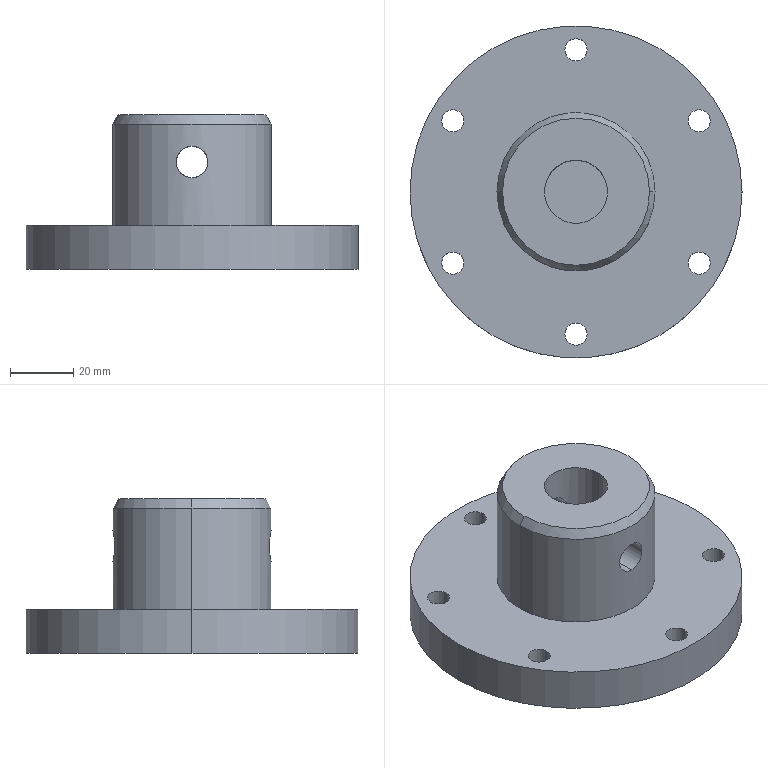Part | SolidWorks | features ICE 2, Chamfer 1, Extrusion 1 | 1 solid | 28 faces | box 105 x 105 x 49 mm | volume 172934 mm3 | cylinder 22 | plane 4 | cone 2 | commonest cylinder face diameters 7 x12 10 x4 20 x2 50 x2 105 x2
STEP:
#1=CARTESIAN_POINT('',(23.268,0.,49.));
#2=VERTEX_POINT('',#1);
#3=CARTESIAN_POINT('',(-23.268,0.,49.));
#4=VERTEX_POINT('',#3);
#5=CARTESIAN_POINT('',(0.,0.,49.));
#6=DIRECTION('',(0.,0.,1.));
#7=DIRECTION('',(1.,0.,0.));
#8=AXIS2_PLACEMENT_3D('',#5,#6,#7);
#9=CIRCLE('',#8,23.268);
#10=EDGE_CURVE('',#2,#4,#9,.T.);
#11=ORIENTED_EDGE('',*,*,#10,.F.);
#12=CARTESIAN_POINT('',(25.,0.,46.));
#13=VERTEX_POINT('',#12);
#14=CARTESIAN_POINT('',(23.268,0.,49.));
#15=DIRECTION('',(0.5,0.,-0.866));
#16=VECTOR('',#15,1000.);
#17=LINE('',#14,#16);
#18=EDGE_CURVE('',#2,#13,#17,.T.);
#19=ORIENTED_EDGE('',*,*,#18,.T.);
#20=CARTESIAN_POINT('',(-25.,0.,46.));
#21=VERTEX_POINT('',#20);
#22=CARTESIAN_POINT('',(0.,0.,46.));
#23=DIRECTION('',(0.,0.,-1.));
#24=DIRECTION('',(1.,0.,0.));
#25=AXIS2_PLACEMENT_3D('',#22,#23,#24);
#26=CIRCLE('',#25,25.);
#27=EDGE_CURVE('',#21,#13,#26,.T.);
#28=ORIENTED_EDGE('',*,*,#27,.F.);
#29=CARTESIAN_POINT('',(-23.268,0.,49.));
#30=DIRECTION('',(-0.5,0.,-0.866));
#31=VECTOR('',#30,1000.);
#32=LINE('',#29,#31);
#33=EDGE_CURVE('',#4,#21,#32,.T.);
#34=ORIENTED_EDGE('',*,*,#33,.F.);
#35=EDGE_LOOP('',(#11,#19,#28,#34));
#36=FACE_OUTER_BOUND('',#35,.T.);
#37=CARTESIAN_POINT('',(0.,0.,49.));
#38=DIRECTION('',(0.,0.,-1.));
#39=DIRECTION('',(-1.,0.,0.));
#40=AXIS2_PLACEMENT_3D('',#37,#38,#39);
#41=CONICAL_SURFACE('',#40,23.268,0.5236);
#42=ADVANCED_FACE('',(#36),#41,.T.);
#43=CARTESIAN_POINT('',(0.,-25.,29.));
#44=VERTEX_POINT('',#43);
#45=CARTESIAN_POINT('',(0.,-25.,39.));
#46=VERTEX_POINT('',#45);
#47=CARTESIAN_POINT('',(0.,-25.,29.));
#48=CARTESIAN_POINT('',(-0.3267,-25.,29.));
#49=CARTESIAN_POINT('',(-0.652,-24.994,29.032));
#50=CARTESIAN_POINT('',(-1.3,-24.968,29.161));
#51=CARTESIAN_POINT('',(-1.614,-24.95,29.256));
#52=CARTESIAN_POINT('',(-2.065,-24.915,29.444));
#53=CARTESIAN_POINT('',(-2.213,-24.902,29.513));
#54=CARTESIAN_POINT('',(-2.502,-24.875,29.668));
#55=CARTESIAN_POINT('',(-2.644,-24.86,29.753));
#56=CARTESIAN_POINT('',(-3.052,-24.815,30.026));
#57=CARTESIAN_POINT('',(-3.303,-24.782,30.232));
#58=CARTESIAN_POINT('',(-3.764,-24.716,30.693));
#59=CARTESIAN_POINT('',(-3.975,-24.683,30.949));
#60=CARTESIAN_POINT('',(-4.337,-24.622,31.49));
#61=CARTESIAN_POINT('',(-4.491,-24.594,31.777));
#62=CARTESIAN_POINT('',(-4.743,-24.546,32.384));
#63=CARTESIAN_POINT('',(-4.839,-24.527,32.7));
#64=CARTESIAN_POINT('',(-4.967,-24.502,33.34));
#65=CARTESIAN_POINT('',(-5.,-24.495,33.667));
#66=CARTESIAN_POINT('',(-5.,-24.495,34.328));
#67=CARTESIAN_POINT('',(-4.968,-24.502,34.653));
#68=CARTESIAN_POINT('',(-4.841,-24.527,35.294));
#69=CARTESIAN_POINT('',(-4.744,-24.546,35.612));
#70=CARTESIAN_POINT('',(-4.494,-24.593,36.216));
#71=CARTESIAN_POINT('',(-4.341,-24.621,36.503));
#72=CARTESIAN_POINT('',(-4.068,-24.667,36.912));
#73=CARTESIAN_POINT('',(-3.97,-24.683,37.045));
#74=CARTESIAN_POINT('',(-3.762,-24.716,37.298));
#75=CARTESIAN_POINT('',(-3.653,-24.732,37.418));
#76=CARTESIAN_POINT('',(-3.308,-24.781,37.763));
#77=CARTESIAN_POINT('',(-3.057,-24.814,37.971));
#78=CARTESIAN_POINT('',(-2.509,-24.875,38.337));
#79=CARTESIAN_POINT('',(-2.222,-24.903,38.491));
#80=CARTESIAN_POINT('',(-1.62,-24.949,38.741));
#81=CARTESIAN_POINT('',(-1.303,-24.968,38.838));
#82=CARTESIAN_POINT('',(-0.658,-24.993,38.967));
#83=CARTESIAN_POINT('',(-0.3312,-25.,39.));
#84=CARTESIAN_POINT('',(0.,-25.,39.));
#85=B_SPLINE_CURVE_WITH_KNOTS('',3,(#47,#48,#49,#50,#51,#52,#53,#54,#55,#56,#57,#58,#59,#60,#61,#62,#63,#64,#65,#66,#67,#68,#69,#70,#71,#72,#73,#74,#75,#76,#77,#78,#79,#80,#81,#82,#83,#84),.UNSPECIFIED.,.F.,.F.,(4,2,2,2,2,2,2,2,2,2,2,2,2,2,2,2,2,2,4),(0.01567,0.01665,0.01763,0.01812,0.01861,0.01959,0.02057,0.02155,0.02253,0.02351,0.02449,0.02546,0.02644,0.02693,0.02742,0.0284,0.02938,0.03036,0.03134),.UNSPECIFIED.);
#86=EDGE_CURVE('',#44,#46,#85,.T.);
#87=ORIENTED_EDGE('',*,*,#86,.F.);
#88=CARTESIAN_POINT('',(0.,-10.,29.));
#89=VERTEX_POINT('',#88);
#90=CARTESIAN_POINT('',(0.,-52.5,29.));
#91=DIRECTION('',(0.,1.,0.));
#92=VECTOR('',#91,1000.);
#93=LINE('',#90,#92);
#94=EDGE_CURVE('',#44,#89,#93,.T.);
#95=ORIENTED_EDGE('',*,*,#94,.T.);
#96=CARTESIAN_POINT('',(0.,-10.,39.));
#97=VERTEX_POINT('',#96);
#98=CARTESIAN_POINT('',(0.,-10.,29.));
#99=CARTESIAN_POINT('',(-0.3314,-10.,29.));
#100=CARTESIAN_POINT('',(-0.6687,-9.983,29.034));
#101=CARTESIAN_POINT('',(-1.317,-9.918,29.165));
#102=CARTESIAN_POINT('',(-1.631,-9.871,29.262));
#103=CARTESIAN_POINT('',(-2.24,-9.751,29.518));
#104=CARTESIAN_POINT('',(-2.526,-9.68,29.673));
#105=CARTESIAN_POINT('',(-3.061,-9.524,30.034));
#106=CARTESIAN_POINT('',(-3.314,-9.438,30.242));
#107=CARTESIAN_POINT('',(-3.767,-9.266,30.697));
#108=CARTESIAN_POINT('',(-3.971,-9.18,30.944));
#109=CARTESIAN_POINT('',(-4.331,-9.016,31.48));
#110=CARTESIAN_POINT('',(-4.487,-8.938,31.769));
#111=CARTESIAN_POINT('',(-4.737,-8.808,32.367));
#112=CARTESIAN_POINT('',(-4.834,-8.754,32.679));
#113=CARTESIAN_POINT('',(-4.933,-8.699,33.168));
#114=CARTESIAN_POINT('',(-4.958,-8.684,33.334));
#115=CARTESIAN_POINT('',(-4.991,-8.665,33.664));
#116=CARTESIAN_POINT('',(-5.008,-8.656,33.994));
#117=CARTESIAN_POINT('',(-4.992,-8.665,34.325));
#118=CARTESIAN_POINT('',(-4.959,-8.684,34.657));
#119=CARTESIAN_POINT('',(-4.935,-8.698,34.823));
#120=CARTESIAN_POINT('',(-4.836,-8.753,35.311));
#121=CARTESIAN_POINT('',(-4.74,-8.806,35.625));
#122=CARTESIAN_POINT('',(-4.487,-8.938,36.23));
#123=CARTESIAN_POINT('',(-4.332,-9.015,36.518));
#124=CARTESIAN_POINT('',(-3.973,-9.179,37.053));
#125=CARTESIAN_POINT('',(-3.767,-9.267,37.304));
#126=CARTESIAN_POINT('',(-3.311,-9.439,37.761));
#127=CARTESIAN_POINT('',(-3.064,-9.523,37.965));
#128=CARTESIAN_POINT('',(-2.528,-9.679,38.326));
#129=CARTESIAN_POINT('',(-2.237,-9.751,38.483));
#130=CARTESIAN_POINT('',(-1.635,-9.87,38.736));
#131=CARTESIAN_POINT('',(-1.323,-9.918,38.833));
#132=CARTESIAN_POINT('',(-0.6735,-9.983,38.965));
#133=CARTESIAN_POINT('',(-0.3359,-10.,39.));
#134=CARTESIAN_POINT('',(0.,-10.,39.));
#135=B_SPLINE_CURVE_WITH_KNOTS('',3,(#98,#99,#100,#101,#102,#103,#104,#105,#106,#107,#108,#109,#110,#111,#112,#113,#114,#115,#116,#117,#118,#119,#120,#121,#122,#123,#124,#125,#126,#127,#128,#129,#130,#131,#132,#133,#134),.UNSPECIFIED.,.F.,.F.,(4,2,2,2,2,2,2,2,2,1,2,2,2,2,2,2,2,2,4),(0.0159,0.0169,0.01789,0.01888,0.01987,0.02087,0.02186,0.02285,0.02335,0.02384,0.02434,0.02484,0.02583,0.02682,0.02781,0.02881,0.0298,0.03079,0.03178),.UNSPECIFIED.);
#136=EDGE_CURVE('',#89,#97,#135,.T.);
#137=ORIENTED_EDGE('',*,*,#136,.T.);
#138=CARTESIAN_POINT('',(0.,-52.5,39.));
#139=DIRECTION('',(0.,1.,0.));
#140=VECTOR('',#139,1000.);
#141=LINE('',#138,#140);
#142=EDGE_CURVE('',#46,#97,#141,.T.);
#143=ORIENTED_EDGE('',*,*,#142,.F.);
#144=EDGE_LOOP('',(#87,#95,#137,#143));
#145=FACE_OUTER_BOUND('',#144,.T.);
#146=CARTESIAN_POINT('',(0.,-52.5,34.));
#147=DIRECTION('',(0.,1.,0.));
#148=DIRECTION('',(0.,0.,1.));
#149=AXIS2_PLACEMENT_3D('',#146,#147,#148);
#150=CYLINDRICAL_SURFACE('',#149,5.);
#151=ADVANCED_FACE('',(#145),#150,.F.);
#152=CARTESIAN_POINT('',(0.,10.,39.));
#153=VERTEX_POINT('',#152);
#154=CARTESIAN_POINT('',(0.,10.,29.));
#155=VERTEX_POINT('',#154);
#156=CARTESIAN_POINT('',(0.,10.,39.));
#157=CARTESIAN_POINT('',(-0.3365,10.,39.));
#158=CARTESIAN_POINT('',(-0.6663,9.983,38.966));
#159=CARTESIAN_POINT('',(-1.314,9.919,38.836));
#160=CARTESIAN_POINT('',(-1.634,9.87,38.737));
#161=CARTESIAN_POINT('',(-2.238,9.751,38.483));
#162=CARTESIAN_POINT('',(-2.523,9.68,38.329));
#163=CARTESIAN_POINT('',(-3.063,9.524,37.965));
#164=CARTESIAN_POINT('',(-3.313,9.438,37.758));
#165=CARTESIAN_POINT('',(-3.766,9.267,37.305));
#166=CARTESIAN_POINT('',(-3.972,9.179,37.054));
#167=CARTESIAN_POINT('',(-4.333,9.015,36.516));
#168=CARTESIAN_POINT('',(-4.486,8.939,36.232));
#169=CARTESIAN_POINT('',(-4.674,8.841,35.783));
#170=CARTESIAN_POINT('',(-4.73,8.811,35.629));
#171=CARTESIAN_POINT('',(-4.827,8.758,35.313));
#172=CARTESIAN_POINT('',(-4.868,8.735,35.152));
#173=CARTESIAN_POINT('',(-4.966,8.68,34.666));
#174=CARTESIAN_POINT('',(-5.,8.66,34.338));
#175=CARTESIAN_POINT('',(-5.,8.66,33.838));
#176=CARTESIAN_POINT('',(-4.992,8.665,33.67));
#177=CARTESIAN_POINT('',(-4.959,8.684,33.337));
#178=CARTESIAN_POINT('',(-4.934,8.698,33.173));
#179=CARTESIAN_POINT('',(-4.836,8.753,32.688));
#180=CARTESIAN_POINT('',(-4.738,8.807,32.37));
#181=CARTESIAN_POINT('',(-4.485,8.939,31.765));
#182=CARTESIAN_POINT('',(-4.331,9.016,31.48));
#183=CARTESIAN_POINT('',(-3.97,9.18,30.943));
#184=CARTESIAN_POINT('',(-3.763,9.268,30.692));
#185=CARTESIAN_POINT('',(-3.309,9.44,30.238));
#186=CARTESIAN_POINT('',(-3.061,9.524,30.033));
#187=CARTESIAN_POINT('',(-2.52,9.681,29.669));
#188=CARTESIAN_POINT('',(-2.233,9.752,29.514));
#189=CARTESIAN_POINT('',(-1.783,9.841,29.326));
#190=CARTESIAN_POINT('',(-1.629,9.868,29.27));
#191=CARTESIAN_POINT('',(-1.314,9.915,29.173));
#192=CARTESIAN_POINT('',(-1.152,9.935,29.132));
#193=CARTESIAN_POINT('',(-0.6614,9.984,29.033));
#194=CARTESIAN_POINT('',(-0.332,10.,29.));
#195=CARTESIAN_POINT('',(0.,10.,29.));
#196=B_SPLINE_CURVE_WITH_KNOTS('',3,(#156,#157,#158,#159,#160,#161,#162,#163,#164,#165,#166,#167,#168,#169,#170,#171,#172,#173,#174,#175,#176,#177,#178,#179,#180,#181,#182,#183,#184,#185,#186,#187,#188,#189,#190,#191,#192,#193,#194,#195),.UNSPECIFIED.,.F.,.F.,(4,2,2,2,2,2,2,2,2,2,2,2,2,2,2,2,2,2,2,4),(0.,0.0009941,0.001988,0.002982,0.003976,0.00497,0.005964,0.006461,0.006958,0.007952,0.008449,0.008947,0.009941,0.01093,0.01193,0.01292,0.01392,0.01441,0.01491,0.0159),.UNSPECIFIED.);
#197=EDGE_CURVE('',#153,#155,#196,.T.);
#198=ORIENTED_EDGE('',*,*,#197,.T.);
#199=CARTESIAN_POINT('',(0.,25.,29.));
#200=VERTEX_POINT('',#199);
#201=CARTESIAN_POINT('',(0.,-52.5,29.));
#202=DIRECTION('',(0.,1.,0.));
#203=VECTOR('',#202,1000.);
#204=LINE('',#201,#203);
#205=EDGE_CURVE('',#155,#200,#204,.T.);
#206=ORIENTED_EDGE('',*,*,#205,.T.);
#207=CARTESIAN_POINT('',(0.,25.,39.));
#208=VERTEX_POINT('',#207);
#209=CARTESIAN_POINT('',(0.,25.,39.));
#210=CARTESIAN_POINT('',(-0.3313,25.,39.));
#211=CARTESIAN_POINT('',(-0.6568,24.993,38.967));
#212=CARTESIAN_POINT('',(-1.297,24.968,38.84));
#213=CARTESIAN_POINT('',(-1.615,24.95,38.743));
#214=CARTESIAN_POINT('',(-2.22,24.903,38.492));
#215=CARTESIAN_POINT('',(-2.507,24.875,38.338));
#216=CARTESIAN_POINT('',(-3.05,24.815,37.975));
#217=CARTESIAN_POINT('',(-3.306,24.781,37.765));
#218=CARTESIAN_POINT('',(-3.766,24.716,37.305));
#219=CARTESIAN_POINT('',(-3.973,24.683,37.053));
#220=CARTESIAN_POINT('',(-4.339,24.621,36.507));
#221=CARTESIAN_POINT('',(-4.493,24.593,36.217));
#222=CARTESIAN_POINT('',(-4.743,24.546,35.616));
#223=CARTESIAN_POINT('',(-4.839,24.527,35.3));
#224=CARTESIAN_POINT('',(-4.968,24.502,34.654));
#225=CARTESIAN_POINT('',(-5.,24.495,34.329));
#226=CARTESIAN_POINT('',(-5.,24.495,33.675));
#227=CARTESIAN_POINT('',(-4.967,24.502,33.343));
#228=CARTESIAN_POINT('',(-4.839,24.527,32.701));
#229=CARTESIAN_POINT('',(-4.745,24.546,32.389));
#230=CARTESIAN_POINT('',(-4.556,24.581,31.934));
#231=CARTESIAN_POINT('',(-4.485,24.595,31.784));
#232=CARTESIAN_POINT('',(-4.33,24.622,31.495));
#233=CARTESIAN_POINT('',(-4.247,24.637,31.356));
#234=CARTESIAN_POINT('',(-3.975,24.683,30.95));
#235=CARTESIAN_POINT('',(-3.768,24.716,30.697));
#236=CARTESIAN_POINT('',(-3.303,24.782,30.232));
#237=CARTESIAN_POINT('',(-3.051,24.815,30.026));
#238=CARTESIAN_POINT('',(-2.51,24.875,29.664));
#239=CARTESIAN_POINT('',(-2.218,24.903,29.507));
#240=CARTESIAN_POINT('',(-1.613,24.95,29.256));
#241=CARTESIAN_POINT('',(-1.301,24.968,29.161));
#242=CARTESIAN_POINT('',(-0.6587,24.993,29.033));
#243=CARTESIAN_POINT('',(-0.3268,25.,29.));
#244=CARTESIAN_POINT('',(0.,25.,29.));
#245=B_SPLINE_CURVE_WITH_KNOTS('',3,(#209,#210,#211,#212,#213,#214,#215,#216,#217,#218,#219,#220,#221,#222,#223,#224,#225,#226,#227,#228,#229,#230,#231,#232,#233,#234,#235,#236,#237,#238,#239,#240,#241,#242,#243,#244),.UNSPECIFIED.,.F.,.F.,(4,2,2,2,2,2,2,2,2,2,2,2,2,2,2,2,2,4),(0.,0.0009795,0.001959,0.002938,0.003918,0.004897,0.005877,0.006856,0.007836,0.008815,0.009795,0.01028,0.01077,0.01175,0.01273,0.01371,0.01469,0.01567),.UNSPECIFIED.);
#246=EDGE_CURVE('',#208,#200,#245,.T.);
#247=ORIENTED_EDGE('',*,*,#246,.F.);
#248=CARTESIAN_POINT('',(0.,-52.5,39.));
#249=DIRECTION('',(0.,1.,0.));
#250=VECTOR('',#249,1000.);
#251=LINE('',#248,#250);
#252=EDGE_CURVE('',#153,#208,#251,.T.);
#253=ORIENTED_EDGE('',*,*,#252,.F.);
#254=EDGE_LOOP('',(#198,#206,#247,#253));
#255=FACE_OUTER_BOUND('',#254,.T.);
#256=CARTESIAN_POINT('',(0.,-52.5,34.));
#257=DIRECTION('',(0.,1.,0.));
#258=DIRECTION('',(0.,0.,1.));
#259=AXIS2_PLACEMENT_3D('',#256,#257,#258);
#260=CYLINDRICAL_SURFACE('',#259,5.);
#261=ADVANCED_FACE('',(#255),#260,.F.);
#262=CARTESIAN_POINT('',(0.,-10.,39.));
#263=CARTESIAN_POINT('',(0.3365,-10.,39.));
#264=CARTESIAN_POINT('',(0.6663,-9.983,38.966));
#265=CARTESIAN_POINT('',(1.314,-9.919,38.836));
#266=CARTESIAN_POINT('',(1.634,-9.87,38.737));
#267=CARTESIAN_POINT('',(2.238,-9.751,38.483));
#268=CARTESIAN_POINT('',(2.523,-9.68,38.329));
#269=CARTESIAN_POINT('',(3.063,-9.524,37.965));
#270=CARTESIAN_POINT('',(3.313,-9.438,37.758));
#271=CARTESIAN_POINT('',(3.766,-9.267,37.305));
#272=CARTESIAN_POINT('',(3.972,-9.179,37.054));
#273=CARTESIAN_POINT('',(4.333,-9.015,36.516));
#274=CARTESIAN_POINT('',(4.486,-8.939,36.232));
#275=CARTESIAN_POINT('',(4.674,-8.841,35.783));
#276=CARTESIAN_POINT('',(4.73,-8.811,35.629));
#277=CARTESIAN_POINT('',(4.827,-8.758,35.313));
#278=CARTESIAN_POINT('',(4.868,-8.735,35.152));
#279=CARTESIAN_POINT('',(4.966,-8.68,34.666));
#280=CARTESIAN_POINT('',(5.,-8.66,34.338));
#281=CARTESIAN_POINT('',(5.,-8.66,33.838));
#282=CARTESIAN_POINT('',(4.992,-8.665,33.67));
#283=CARTESIAN_POINT('',(4.959,-8.684,33.337));
#284=CARTESIAN_POINT('',(4.934,-8.698,33.173));
#285=CARTESIAN_POINT('',(4.836,-8.753,32.688));
#286=CARTESIAN_POINT('',(4.738,-8.807,32.37));
#287=CARTESIAN_POINT('',(4.485,-8.939,31.765));
#288=CARTESIAN_POINT('',(4.331,-9.016,31.48));
#289=CARTESIAN_POINT('',(3.97,-9.18,30.943));
#290=CARTESIAN_POINT('',(3.763,-9.268,30.692));
#291=CARTESIAN_POINT('',(3.309,-9.44,30.238));
#292=CARTESIAN_POINT('',(3.061,-9.524,30.033));
#293=CARTESIAN_POINT('',(2.52,-9.681,29.669));
#294=CARTESIAN_POINT('',(2.233,-9.752,29.514));
#295=CARTESIAN_POINT('',(1.783,-9.841,29.326));
#296=CARTESIAN_POINT('',(1.629,-9.868,29.27));
#297=CARTESIAN_POINT('',(1.314,-9.915,29.173));
#298=CARTESIAN_POINT('',(1.152,-9.935,29.132));
#299=CARTESIAN_POINT('',(0.6614,-9.984,29.033));
#300=CARTESIAN_POINT('',(0.332,-10.,29.));
#301=CARTESIAN_POINT('',(0.,-10.,29.));
#302=B_SPLINE_CURVE_WITH_KNOTS('',3,(#262,#263,#264,#265,#266,#267,#268,#269,#270,#271,#272,#273,#274,#275,#276,#277,#278,#279,#280,#281,#282,#283,#284,#285,#286,#287,#288,#289,#290,#291,#292,#293,#294,#295,#296,#297,#298,#299,#300,#301),.UNSPECIFIED.,.F.,.F.,(4,2,2,2,2,2,2,2,2,2,2,2,2,2,2,2,2,2,2,4),(0.,0.0009941,0.001988,0.002982,0.003976,0.00497,0.005964,0.006461,0.006958,0.007952,0.008449,0.008947,0.009941,0.01093,0.01193,0.01292,0.01392,0.01441,0.01491,0.0159),.UNSPECIFIED.);
#303=EDGE_CURVE('',#97,#89,#302,.T.);
#304=ORIENTED_EDGE('',*,*,#303,.F.);
#305=ORIENTED_EDGE('',*,*,#136,.F.);
#306=EDGE_LOOP('',(#304,#305));
#307=FACE_BOUND('',#306,.T.);
#308=CARTESIAN_POINT('',(-10.,0.,49.));
#309=VERTEX_POINT('',#308);
#310=CARTESIAN_POINT('',(10.,0.,49.));
#311=VERTEX_POINT('',#310);
#312=CARTESIAN_POINT('',(0.,0.,49.));
#313=DIRECTION('',(0.,0.,1.));
#314=DIRECTION('',(1.,0.,0.));
#315=AXIS2_PLACEMENT_3D('',#312,#313,#314);
#316=CIRCLE('',#315,10.);
#317=EDGE_CURVE('',#309,#311,#316,.T.);
#318=ORIENTED_EDGE('',*,*,#317,.T.);
#319=CARTESIAN_POINT('',(10.,0.,14.));
#320=VERTEX_POINT('',#319);
#321=CARTESIAN_POINT('',(10.,0.,49.));
#322=DIRECTION('',(0.,0.,-1.));
#323=VECTOR('',#322,1000.);
#324=LINE('',#321,#323);
#325=EDGE_CURVE('',#311,#320,#324,.T.);
#326=ORIENTED_EDGE('',*,*,#325,.T.);
#327=CARTESIAN_POINT('',(-10.,0.,14.));
#328=VERTEX_POINT('',#327);
#329=CARTESIAN_POINT('',(0.,0.,14.));
#330=DIRECTION('',(0.,0.,-1.));
#331=DIRECTION('',(1.,0.,0.));
#332=AXIS2_PLACEMENT_3D('',#329,#330,#331);
#333=CIRCLE('',#332,10.);
#334=EDGE_CURVE('',#320,#328,#333,.T.);
#335=ORIENTED_EDGE('',*,*,#334,.T.);
#336=CARTESIAN_POINT('',(-10.,0.,49.));
#337=DIRECTION('',(0.,0.,-1.));
#338=VECTOR('',#337,1000.);
#339=LINE('',#336,#338);
#340=EDGE_CURVE('',#309,#328,#339,.T.);
#341=ORIENTED_EDGE('',*,*,#340,.F.);
#342=EDGE_LOOP('',(#318,#326,#335,#341));
#343=FACE_OUTER_BOUND('',#342,.T.);
#344=CARTESIAN_POINT('',(0.,0.,49.));
#345=DIRECTION('',(0.,0.,-1.));
#346=DIRECTION('',(-1.,0.,0.));
#347=AXIS2_PLACEMENT_3D('',#344,#345,#346);
#348=CYLINDRICAL_SURFACE('',#347,10.);
#349=ADVANCED_FACE('',(#307,#343),#348,.F.);
#350=ORIENTED_EDGE('',*,*,#246,.T.);
#351=CARTESIAN_POINT('',(0.,25.,29.));
#352=CARTESIAN_POINT('',(0.3267,25.,29.));
#353=CARTESIAN_POINT('',(0.652,24.994,29.032));
#354=CARTESIAN_POINT('',(1.3,24.968,29.161));
#355=CARTESIAN_POINT('',(1.614,24.95,29.256));
#356=CARTESIAN_POINT('',(2.065,24.915,29.444));
#357=CARTESIAN_POINT('',(2.213,24.902,29.513));
#358=CARTESIAN_POINT('',(2.502,24.875,29.668));
#359=CARTESIAN_POINT('',(2.644,24.86,29.753));
#360=CARTESIAN_POINT('',(3.052,24.815,30.026));
#361=CARTESIAN_POINT('',(3.303,24.782,30.232));
#362=CARTESIAN_POINT('',(3.764,24.716,30.693));
#363=CARTESIAN_POINT('',(3.975,24.683,30.949));
#364=CARTESIAN_POINT('',(4.337,24.622,31.49));
#365=CARTESIAN_POINT('',(4.491,24.594,31.777));
#366=CARTESIAN_POINT('',(4.743,24.546,32.384));
#367=CARTESIAN_POINT('',(4.839,24.527,32.7));
#368=CARTESIAN_POINT('',(4.967,24.502,33.34));
#369=CARTESIAN_POINT('',(5.,24.495,33.667));
#370=CARTESIAN_POINT('',(5.,24.495,34.328));
#371=CARTESIAN_POINT('',(4.968,24.502,34.653));
#372=CARTESIAN_POINT('',(4.841,24.527,35.294));
#373=CARTESIAN_POINT('',(4.744,24.546,35.612));
#374=CARTESIAN_POINT('',(4.494,24.593,36.216));
#375=CARTESIAN_POINT('',(4.341,24.621,36.503));
#376=CARTESIAN_POINT('',(4.068,24.667,36.912));
#377=CARTESIAN_POINT('',(3.97,24.683,37.045));
#378=CARTESIAN_POINT('',(3.762,24.716,37.298));
#379=CARTESIAN_POINT('',(3.653,24.732,37.418));
#380=CARTESIAN_POINT('',(3.308,24.781,37.763));
#381=CARTESIAN_POINT('',(3.057,24.814,37.971));
#382=CARTESIAN_POINT('',(2.509,24.875,38.337));
#383=CARTESIAN_POINT('',(2.222,24.903,38.491));
#384=CARTESIAN_POINT('',(1.62,24.949,38.741));
#385=CARTESIAN_POINT('',(1.303,24.968,38.838));
#386=CARTESIAN_POINT('',(0.658,24.993,38.967));
#387=CARTESIAN_POINT('',(0.3312,25.,39.));
#388=CARTESIAN_POINT('',(0.,25.,39.));
#389=B_SPLINE_CURVE_WITH_KNOTS('',3,(#351,#352,#353,#354,#355,#356,#357,#358,#359,#360,#361,#362,#363,#364,#365,#366,#367,#368,#369,#370,#371,#372,#373,#374,#375,#376,#377,#378,#379,#380,#381,#382,#383,#384,#385,#386,#387,#388),.UNSPECIFIED.,.F.,.F.,(4,2,2,2,2,2,2,2,2,2,2,2,2,2,2,2,2,2,4),(0.01567,0.01665,0.01763,0.01812,0.01861,0.01959,0.02057,0.02155,0.02253,0.02351,0.02449,0.02546,0.02644,0.02693,0.02742,0.0284,0.02938,0.03036,0.03134),.UNSPECIFIED.);
#390=EDGE_CURVE('',#200,#208,#389,.T.);
#391=ORIENTED_EDGE('',*,*,#390,.T.);
#392=EDGE_LOOP('',(#350,#391));
#393=FACE_BOUND('',#392,.T.);
#394=ORIENTED_EDGE('',*,*,#27,.T.);
#395=CARTESIAN_POINT('',(25.,0.,14.));
#396=VERTEX_POINT('',#395);
#397=CARTESIAN_POINT('',(25.,0.,49.));
#398=DIRECTION('',(0.,0.,-1.));
#399=VECTOR('',#398,1000.);
#400=LINE('',#397,#399);
#401=EDGE_CURVE('',#13,#396,#400,.T.);
#402=ORIENTED_EDGE('',*,*,#401,.T.);
#403=CARTESIAN_POINT('',(-25.,0.,14.));
#404=VERTEX_POINT('',#403);
#405=CARTESIAN_POINT('',(0.,0.,14.));
#406=DIRECTION('',(0.,0.,1.));
#407=DIRECTION('',(1.,0.,0.));
#408=AXIS2_PLACEMENT_3D('',#405,#406,#407);
#409=CIRCLE('',#408,25.);
#410=EDGE_CURVE('',#396,#404,#409,.T.);
#411=ORIENTED_EDGE('',*,*,#410,.T.);
#412=CARTESIAN_POINT('',(-25.,0.,49.));
#413=DIRECTION('',(0.,0.,-1.));
#414=VECTOR('',#413,1000.);
#415=LINE('',#412,#414);
#416=EDGE_CURVE('',#21,#404,#415,.T.);
#417=ORIENTED_EDGE('',*,*,#416,.F.);
#418=EDGE_LOOP('',(#394,#402,#411,#417));
#419=FACE_OUTER_BOUND('',#418,.T.);
#420=CARTESIAN_POINT('',(0.,0.,49.));
#421=DIRECTION('',(0.,0.,-1.));
#422=DIRECTION('',(-1.,0.,0.));
#423=AXIS2_PLACEMENT_3D('',#420,#421,#422);
#424=CYLINDRICAL_SURFACE('',#423,25.);
#425=ADVANCED_FACE('',(#393,#419),#424,.T.);
#426=CARTESIAN_POINT('',(-42.471,22.5,14.));
#427=VERTEX_POINT('',#426);
#428=CARTESIAN_POINT('',(-35.471,22.5,14.));
#429=VERTEX_POINT('',#428);
#430=CARTESIAN_POINT('',(-38.971,22.5,14.));
#431=DIRECTION('',(0.,0.,1.));
#432=DIRECTION('',(1.,0.,0.));
#433=AXIS2_PLACEMENT_3D('',#430,#431,#432);
#434=CIRCLE('',#433,3.5);
#435=EDGE_CURVE('',#427,#429,#434,.T.);
#436=ORIENTED_EDGE('',*,*,#435,.T.);
#437=CARTESIAN_POINT('',(-35.471,22.5,0.));
#438=VERTEX_POINT('',#437);
#439=CARTESIAN_POINT('',(-35.471,22.5,14.));
#440=DIRECTION('',(0.,0.,-1.));
#441=VECTOR('',#440,1000.);
#442=LINE('',#439,#441);
#443=EDGE_CURVE('',#429,#438,#442,.T.);
#444=ORIENTED_EDGE('',*,*,#443,.T.);
#445=CARTESIAN_POINT('',(-42.471,22.5,0.));
#446=VERTEX_POINT('',#445);
#447=CARTESIAN_POINT('',(-38.971,22.5,0.));
#448=DIRECTION('',(0.,0.,1.));
#449=DIRECTION('',(1.,0.,0.));
#450=AXIS2_PLACEMENT_3D('',#447,#448,#449);
#451=CIRCLE('',#450,3.5);
#452=EDGE_CURVE('',#446,#438,#451,.T.);
#453=ORIENTED_EDGE('',*,*,#452,.F.);
#454=CARTESIAN_POINT('',(-42.471,22.5,14.));
#455=DIRECTION('',(0.,0.,-1.));
#456=VECTOR('',#455,1000.);
#457=LINE('',#454,#456);
#458=EDGE_CURVE('',#427,#446,#457,.T.);
#459=ORIENTED_EDGE('',*,*,#458,.F.);
#460=EDGE_LOOP('',(#436,#444,#453,#459));
#461=FACE_OUTER_BOUND('',#460,.T.);
#462=CARTESIAN_POINT('',(-38.971,22.5,14.));
#463=DIRECTION('',(0.,0.,-1.));
#464=DIRECTION('',(-1.,0.,0.));
#465=AXIS2_PLACEMENT_3D('',#462,#463,#464);
#466=CYLINDRICAL_SURFACE('',#465,3.5);
#467=ADVANCED_FACE('',(#461),#466,.F.);
#468=CARTESIAN_POINT('',(-42.471,-22.5,14.));
#469=VERTEX_POINT('',#468);
#470=CARTESIAN_POINT('',(-35.471,-22.5,14.));
#471=VERTEX_POINT('',#470);
#472=CARTESIAN_POINT('',(-38.971,-22.5,14.));
#473=DIRECTION('',(0.,0.,1.));
#474=DIRECTION('',(1.,0.,0.));
#475=AXIS2_PLACEMENT_3D('',#472,#473,#474);
#476=CIRCLE('',#475,3.5);
#477=EDGE_CURVE('',#469,#471,#476,.T.);
#478=ORIENTED_EDGE('',*,*,#477,.T.);
#479=CARTESIAN_POINT('',(-35.471,-22.5,0.));
#480=VERTEX_POINT('',#479);
#481=CARTESIAN_POINT('',(-35.471,-22.5,14.));
#482=DIRECTION('',(0.,0.,-1.));
#483=VECTOR('',#482,1000.);
#484=LINE('',#481,#483);
#485=EDGE_CURVE('',#471,#480,#484,.T.);
#486=ORIENTED_EDGE('',*,*,#485,.T.);
#487=CARTESIAN_POINT('',(-42.471,-22.5,0.));
#488=VERTEX_POINT('',#487);
#489=CARTESIAN_POINT('',(-38.971,-22.5,0.));
#490=DIRECTION('',(0.,0.,1.));
#491=DIRECTION('',(1.,0.,0.));
#492=AXIS2_PLACEMENT_3D('',#489,#490,#491);
#493=CIRCLE('',#492,3.5);
#494=EDGE_CURVE('',#488,#480,#493,.T.);
#495=ORIENTED_EDGE('',*,*,#494,.F.);
#496=CARTESIAN_POINT('',(-42.471,-22.5,14.));
#497=DIRECTION('',(0.,0.,-1.));
#498=VECTOR('',#497,1000.);
#499=LINE('',#496,#498);
#500=EDGE_CURVE('',#469,#488,#499,.T.);
#501=ORIENTED_EDGE('',*,*,#500,.F.);
#502=EDGE_LOOP('',(#478,#486,#495,#501));
#503=FACE_OUTER_BOUND('',#502,.T.);
#504=CARTESIAN_POINT('',(-38.971,-22.5,14.));
#505=DIRECTION('',(0.,0.,-1.));
#506=DIRECTION('',(-1.,0.,0.));
#507=AXIS2_PLACEMENT_3D('',#504,#505,#506);
#508=CYLINDRICAL_SURFACE('',#507,3.5);
#509=ADVANCED_FACE('',(#503),#508,.F.);
#510=CARTESIAN_POINT('',(-3.5,-45.,14.));
#511=VERTEX_POINT('',#510);
#512=CARTESIAN_POINT('',(3.5,-45.,14.));
#513=VERTEX_POINT('',#512);
#514=CARTESIAN_POINT('',(0.,-45.,14.));
#515=DIRECTION('',(0.,0.,1.));
#516=DIRECTION('',(1.,0.,0.));
#517=AXIS2_PLACEMENT_3D('',#514,#515,#516);
#518=CIRCLE('',#517,3.5);
#519=EDGE_CURVE('',#511,#513,#518,.T.);
#520=ORIENTED_EDGE('',*,*,#519,.T.);
#521=CARTESIAN_POINT('',(3.5,-45.,0.));
#522=VERTEX_POINT('',#521);
#523=CARTESIAN_POINT('',(3.5,-45.,14.));
#524=DIRECTION('',(0.,0.,-1.));
#525=VECTOR('',#524,1000.);
#526=LINE('',#523,#525);
#527=EDGE_CURVE('',#513,#522,#526,.T.);
#528=ORIENTED_EDGE('',*,*,#527,.T.);
#529=CARTESIAN_POINT('',(-3.5,-45.,0.));
#530=VERTEX_POINT('',#529);
#531=CARTESIAN_POINT('',(0.,-45.,0.));
#532=DIRECTION('',(0.,0.,1.));
#533=DIRECTION('',(1.,0.,0.));
#534=AXIS2_PLACEMENT_3D('',#531,#532,#533);
#535=CIRCLE('',#534,3.5);
#536=EDGE_CURVE('',#530,#522,#535,.T.);
#537=ORIENTED_EDGE('',*,*,#536,.F.);
#538=CARTESIAN_POINT('',(-3.5,-45.,14.));
#539=DIRECTION('',(0.,0.,-1.));
#540=VECTOR('',#539,1000.);
#541=LINE('',#538,#540);
#542=EDGE_CURVE('',#511,#530,#541,.T.);
#543=ORIENTED_EDGE('',*,*,#542,.F.);
#544=EDGE_LOOP('',(#520,#528,#537,#543));
#545=FACE_OUTER_BOUND('',#544,.T.);
#546=CARTESIAN_POINT('',(0.,-45.,14.));
#547=DIRECTION('',(0.,0.,-1.));
#548=DIRECTION('',(-1.,0.,0.));
#549=AXIS2_PLACEMENT_3D('',#546,#547,#548);
#550=CYLINDRICAL_SURFACE('',#549,3.5);
#551=ADVANCED_FACE('',(#545),#550,.F.);
#552=CARTESIAN_POINT('',(35.471,-22.5,14.));
#553=VERTEX_POINT('',#552);
#554=CARTESIAN_POINT('',(42.471,-22.5,14.));
#555=VERTEX_POINT('',#554);
#556=CARTESIAN_POINT('',(38.971,-22.5,14.));
#557=DIRECTION('',(0.,0.,1.));
#558=DIRECTION('',(1.,0.,0.));
#559=AXIS2_PLACEMENT_3D('',#556,#557,#558);
#560=CIRCLE('',#559,3.5);
#561=EDGE_CURVE('',#553,#555,#560,.T.);
#562=ORIENTED_EDGE('',*,*,#561,.T.);
#563=CARTESIAN_POINT('',(42.471,-22.5,0.));
#564=VERTEX_POINT('',#563);
#565=CARTESIAN_POINT('',(42.471,-22.5,14.));
#566=DIRECTION('',(0.,0.,-1.));
#567=VECTOR('',#566,1000.);
#568=LINE('',#565,#567);
#569=EDGE_CURVE('',#555,#564,#568,.T.);
#570=ORIENTED_EDGE('',*,*,#569,.T.);
#571=CARTESIAN_POINT('',(35.471,-22.5,0.));
#572=VERTEX_POINT('',#571);
#573=CARTESIAN_POINT('',(38.971,-22.5,0.));
#574=DIRECTION('',(0.,0.,1.));
#575=DIRECTION('',(1.,0.,0.));
#576=AXIS2_PLACEMENT_3D('',#573,#574,#575);
#577=CIRCLE('',#576,3.5);
#578=EDGE_CURVE('',#572,#564,#577,.T.);
#579=ORIENTED_EDGE('',*,*,#578,.F.);
#580=CARTESIAN_POINT('',(35.471,-22.5,14.));
#581=DIRECTION('',(0.,0.,-1.));
#582=VECTOR('',#581,1000.);
#583=LINE('',#580,#582);
#584=EDGE_CURVE('',#553,#572,#583,.T.);
#585=ORIENTED_EDGE('',*,*,#584,.F.);
#586=EDGE_LOOP('',(#562,#570,#579,#585));
#587=FACE_OUTER_BOUND('',#586,.T.);
#588=CARTESIAN_POINT('',(38.971,-22.5,14.));
#589=DIRECTION('',(0.,0.,-1.));
#590=DIRECTION('',(-1.,0.,0.));
#591=AXIS2_PLACEMENT_3D('',#588,#589,#590);
#592=CYLINDRICAL_SURFACE('',#591,3.5);
#593=ADVANCED_FACE('',(#587),#592,.F.);
#594=CARTESIAN_POINT('',(35.471,22.5,14.));
#595=VERTEX_POINT('',#594);
#596=CARTESIAN_POINT('',(42.471,22.5,14.));
#597=VERTEX_POINT('',#596);
#598=CARTESIAN_POINT('',(38.971,22.5,14.));
#599=DIRECTION('',(0.,0.,1.));
#600=DIRECTION('',(1.,0.,0.));
#601=AXIS2_PLACEMENT_3D('',#598,#599,#600);
#602=CIRCLE('',#601,3.5);
#603=EDGE_CURVE('',#595,#597,#602,.T.);
#604=ORIENTED_EDGE('',*,*,#603,.T.);
#605=CARTESIAN_POINT('',(42.471,22.5,0.));
#606=VERTEX_POINT('',#605);
#607=CARTESIAN_POINT('',(42.471,22.5,14.));
#608=DIRECTION('',(0.,0.,-1.));
#609=VECTOR('',#608,1000.);
#610=LINE('',#607,#609);
#611=EDGE_CURVE('',#597,#606,#610,.T.);
#612=ORIENTED_EDGE('',*,*,#611,.T.);
#613=CARTESIAN_POINT('',(35.471,22.5,0.));
#614=VERTEX_POINT('',#613);
#615=CARTESIAN_POINT('',(38.971,22.5,0.));
#616=DIRECTION('',(0.,0.,1.));
#617=DIRECTION('',(1.,0.,0.));
#618=AXIS2_PLACEMENT_3D('',#615,#616,#617);
#619=CIRCLE('',#618,3.5);
#620=EDGE_CURVE('',#614,#606,#619,.T.);
#621=ORIENTED_EDGE('',*,*,#620,.F.);
#622=CARTESIAN_POINT('',(35.471,22.5,14.));
#623=DIRECTION('',(0.,0.,-1.));
#624=VECTOR('',#623,1000.);
#625=LINE('',#622,#624);
#626=EDGE_CURVE('',#595,#614,#625,.T.);
#627=ORIENTED_EDGE('',*,*,#626,.F.);
#628=EDGE_LOOP('',(#604,#612,#621,#627));
#629=FACE_OUTER_BOUND('',#628,.T.);
#630=CARTESIAN_POINT('',(38.971,22.5,14.));
#631=DIRECTION('',(0.,0.,-1.));
#632=DIRECTION('',(-1.,0.,0.));
#633=AXIS2_PLACEMENT_3D('',#630,#631,#632);
#634=CYLINDRICAL_SURFACE('',#633,3.5);
#635=ADVANCED_FACE('',(#629),#634,.F.);
#636=CARTESIAN_POINT('',(-3.5,45.,14.));
#637=VERTEX_POINT('',#636);
#638=CARTESIAN_POINT('',(3.5,45.,14.));
#639=VERTEX_POINT('',#638);
#640=CARTESIAN_POINT('',(0.,45.,14.));
#641=DIRECTION('',(0.,0.,1.));
#642=DIRECTION('',(1.,0.,0.));
#643=AXIS2_PLACEMENT_3D('',#640,#641,#642);
#644=CIRCLE('',#643,3.5);
#645=EDGE_CURVE('',#637,#639,#644,.T.);
#646=ORIENTED_EDGE('',*,*,#645,.T.);
#647=CARTESIAN_POINT('',(3.5,45.,0.));
#648=VERTEX_POINT('',#647);
#649=CARTESIAN_POINT('',(3.5,45.,14.));
#650=DIRECTION('',(0.,0.,-1.));
#651=VECTOR('',#650,1000.);
#652=LINE('',#649,#651);
#653=EDGE_CURVE('',#639,#648,#652,.T.);
#654=ORIENTED_EDGE('',*,*,#653,.T.);
#655=CARTESIAN_POINT('',(-3.5,45.,0.));
#656=VERTEX_POINT('',#655);
#657=CARTESIAN_POINT('',(0.,45.,0.));
#658=DIRECTION('',(0.,0.,1.));
#659=DIRECTION('',(1.,0.,0.));
#660=AXIS2_PLACEMENT_3D('',#657,#658,#659);
#661=CIRCLE('',#660,3.5);
#662=EDGE_CURVE('',#656,#648,#661,.T.);
#663=ORIENTED_EDGE('',*,*,#662,.F.);
#664=CARTESIAN_POINT('',(-3.5,45.,14.));
#665=DIRECTION('',(0.,0.,-1.));
#666=VECTOR('',#665,1000.);
#667=LINE('',#664,#666);
#668=EDGE_CURVE('',#637,#656,#667,.T.);
#669=ORIENTED_EDGE('',*,*,#668,.F.);
#670=EDGE_LOOP('',(#646,#654,#663,#669));
#671=FACE_OUTER_BOUND('',#670,.T.);
#672=CARTESIAN_POINT('',(0.,45.,14.));
#673=DIRECTION('',(0.,0.,-1.));
#674=DIRECTION('',(-1.,0.,0.));
#675=AXIS2_PLACEMENT_3D('',#672,#673,#674);
#676=CYLINDRICAL_SURFACE('',#675,3.5);
#677=ADVANCED_FACE('',(#671),#676,.F.);
#678=CARTESIAN_POINT('',(52.5,0.,14.));
#679=VERTEX_POINT('',#678);
#680=CARTESIAN_POINT('',(-52.5,0.,14.));
#681=VERTEX_POINT('',#680);
#682=CARTESIAN_POINT('',(0.,0.,14.));
#683=DIRECTION('',(0.,0.,1.));
#684=DIRECTION('',(1.,0.,0.));
#685=AXIS2_PLACEMENT_3D('',#682,#683,#684);
#686=CIRCLE('',#685,52.5);
#687=EDGE_CURVE('',#679,#681,#686,.T.);
#688=ORIENTED_EDGE('',*,*,#687,.F.);
#689=CARTESIAN_POINT('',(52.5,0.,0.));
#690=VERTEX_POINT('',#689);
#691=CARTESIAN_POINT('',(52.5,0.,14.));
#692=DIRECTION('',(0.,0.,-1.));
#693=VECTOR('',#692,1000.);
#694=LINE('',#691,#693);
#695=EDGE_CURVE('',#679,#690,#694,.T.);
#696=ORIENTED_EDGE('',*,*,#695,.T.);
#697=CARTESIAN_POINT('',(-52.5,0.,0.));
#698=VERTEX_POINT('',#697);
#699=CARTESIAN_POINT('',(0.,0.,0.));
#700=DIRECTION('',(0.,0.,1.));
#701=DIRECTION('',(1.,0.,0.));
#702=AXIS2_PLACEMENT_3D('',#699,#700,#701);
#703=CIRCLE('',#702,52.5);
#704=EDGE_CURVE('',#690,#698,#703,.T.);
#705=ORIENTED_EDGE('',*,*,#704,.T.);
#706=CARTESIAN_POINT('',(-52.5,0.,14.));
#707=DIRECTION('',(0.,0.,-1.));
#708=VECTOR('',#707,1000.);
#709=LINE('',#706,#708);
#710=EDGE_CURVE('',#681,#698,#709,.T.);
#711=ORIENTED_EDGE('',*,*,#710,.F.);
#712=EDGE_LOOP('',(#688,#696,#705,#711));
#713=FACE_OUTER_BOUND('',#712,.T.);
#714=CARTESIAN_POINT('',(0.,0.,14.));
#715=DIRECTION('',(0.,0.,-1.));
#716=DIRECTION('',(-1.,0.,0.));
#717=AXIS2_PLACEMENT_3D('',#714,#715,#716);
#718=CYLINDRICAL_SURFACE('',#717,52.5);
#719=ADVANCED_FACE('',(#713),#718,.T.);
#720=CARTESIAN_POINT('',(0.,0.,14.));
#721=DIRECTION('',(0.,0.,1.));
#722=DIRECTION('',(1.,0.,0.));
#723=AXIS2_PLACEMENT_3D('',#720,#721,#722);
#724=CIRCLE('',#723,25.);
#725=EDGE_CURVE('',#404,#396,#724,.T.);
#726=ORIENTED_EDGE('',*,*,#725,.F.);
#727=ORIENTED_EDGE('',*,*,#410,.F.);
#728=EDGE_LOOP('',(#726,#727));
#729=FACE_BOUND('',#728,.T.);
#730=ORIENTED_EDGE('',*,*,#477,.F.);
#731=CARTESIAN_POINT('',(-38.971,-22.5,14.));
#732=DIRECTION('',(0.,0.,1.));
#733=DIRECTION('',(1.,0.,0.));
#734=AXIS2_PLACEMENT_3D('',#731,#732,#733);
#735=CIRCLE('',#734,3.5);
#736=EDGE_CURVE('',#471,#469,#735,.T.);
#737=ORIENTED_EDGE('',*,*,#736,.F.);
#738=EDGE_LOOP('',(#730,#737));
#739=FACE_BOUND('',#738,.T.);
#740=ORIENTED_EDGE('',*,*,#561,.F.);
#741=CARTESIAN_POINT('',(38.971,-22.5,14.));
#742=DIRECTION('',(0.,0.,1.));
#743=DIRECTION('',(1.,0.,0.));
#744=AXIS2_PLACEMENT_3D('',#741,#742,#743);
#745=CIRCLE('',#744,3.5);
#746=EDGE_CURVE('',#555,#553,#745,.T.);
#747=ORIENTED_EDGE('',*,*,#746,.F.);
#748=EDGE_LOOP('',(#740,#747));
#749=FACE_BOUND('',#748,.T.);
#750=ORIENTED_EDGE('',*,*,#645,.F.);
#751=CARTESIAN_POINT('',(0.,45.,14.));
#752=DIRECTION('',(0.,0.,1.));
#753=DIRECTION('',(1.,0.,0.));
#754=AXIS2_PLACEMENT_3D('',#751,#752,#753);
#755=CIRCLE('',#754,3.5);
#756=EDGE_CURVE('',#639,#637,#755,.T.);
#757=ORIENTED_EDGE('',*,*,#756,.F.);
#758=EDGE_LOOP('',(#750,#757));
#759=FACE_BOUND('',#758,.T.);
#760=CARTESIAN_POINT('',(0.,0.,14.));
#761=DIRECTION('',(0.,0.,1.));
#762=DIRECTION('',(1.,0.,0.));
#763=AXIS2_PLACEMENT_3D('',#760,#761,#762);
#764=CIRCLE('',#763,52.5);
#765=EDGE_CURVE('',#681,#679,#764,.T.);
#766=ORIENTED_EDGE('',*,*,#765,.T.);
#767=ORIENTED_EDGE('',*,*,#687,.T.);
#768=EDGE_LOOP('',(#766,#767));
#769=FACE_OUTER_BOUND('',#768,.T.);
#770=ORIENTED_EDGE('',*,*,#603,.F.);
#771=CARTESIAN_POINT('',(38.971,22.5,14.));
#772=DIRECTION('',(0.,0.,1.));
#773=DIRECTION('',(1.,0.,0.));
#774=AXIS2_PLACEMENT_3D('',#771,#772,#773);
#775=CIRCLE('',#774,3.5);
#776=EDGE_CURVE('',#597,#595,#775,.T.);
#777=ORIENTED_EDGE('',*,*,#776,.F.);
#778=EDGE_LOOP('',(#770,#777));
#779=FACE_BOUND('',#778,.T.);
#780=ORIENTED_EDGE('',*,*,#519,.F.);
#781=CARTESIAN_POINT('',(0.,-45.,14.));
#782=DIRECTION('',(0.,0.,1.));
#783=DIRECTION('',(1.,0.,0.));
#784=AXIS2_PLACEMENT_3D('',#781,#782,#783);
#785=CIRCLE('',#784,3.5);
#786=EDGE_CURVE('',#513,#511,#785,.T.);
#787=ORIENTED_EDGE('',*,*,#786,.F.);
#788=EDGE_LOOP('',(#780,#787));
#789=FACE_BOUND('',#788,.T.);
#790=ORIENTED_EDGE('',*,*,#435,.F.);
#791=CARTESIAN_POINT('',(-38.971,22.5,14.));
#792=DIRECTION('',(0.,0.,1.));
#793=DIRECTION('',(1.,0.,0.));
#794=AXIS2_PLACEMENT_3D('',#791,#792,#793);
#795=CIRCLE('',#794,3.5);
#796=EDGE_CURVE('',#429,#427,#795,.T.);
#797=ORIENTED_EDGE('',*,*,#796,.F.);
#798=EDGE_LOOP('',(#790,#797));
#799=FACE_BOUND('',#798,.T.);
#800=CARTESIAN_POINT('',(0.,0.,14.));
#801=DIRECTION('',(0.,0.,1.));
#802=DIRECTION('',(1.,0.,0.));
#803=AXIS2_PLACEMENT_3D('',#800,#801,#802);
#804=PLANE('',#803);
#805=ADVANCED_FACE('',(#729,#739,#749,#759,#769,#779,#789,#799),#804,.T.);
#806=CARTESIAN_POINT('',(0.,0.,0.));
#807=DIRECTION('',(0.,0.,1.));
#808=DIRECTION('',(1.,0.,0.));
#809=AXIS2_PLACEMENT_3D('',#806,#807,#808);
#810=CIRCLE('',#809,52.5);
#811=EDGE_CURVE('',#698,#690,#810,.T.);
#812=ORIENTED_EDGE('',*,*,#811,.F.);
#813=ORIENTED_EDGE('',*,*,#704,.F.);
#814=EDGE_LOOP('',(#812,#813));
#815=FACE_OUTER_BOUND('',#814,.T.);
#816=ORIENTED_EDGE('',*,*,#662,.T.);
#817=CARTESIAN_POINT('',(0.,45.,0.));
#818=DIRECTION('',(0.,0.,1.));
#819=DIRECTION('',(1.,0.,0.));
#820=AXIS2_PLACEMENT_3D('',#817,#818,#819);
#821=CIRCLE('',#820,3.5);
#822=EDGE_CURVE('',#648,#656,#821,.T.);
#823=ORIENTED_EDGE('',*,*,#822,.T.);
#824=EDGE_LOOP('',(#816,#823));
#825=FACE_BOUND('',#824,.T.);
#826=ORIENTED_EDGE('',*,*,#620,.T.);
#827=CARTESIAN_POINT('',(38.971,22.5,0.));
#828=DIRECTION('',(0.,0.,1.));
#829=DIRECTION('',(1.,0.,0.));
#830=AXIS2_PLACEMENT_3D('',#827,#828,#829);
#831=CIRCLE('',#830,3.5);
#832=EDGE_CURVE('',#606,#614,#831,.T.);
#833=ORIENTED_EDGE('',*,*,#832,.T.);
#834=EDGE_LOOP('',(#826,#833));
#835=FACE_BOUND('',#834,.T.);
#836=ORIENTED_EDGE('',*,*,#578,.T.);
#837=CARTESIAN_POINT('',(38.971,-22.5,0.));
#838=DIRECTION('',(0.,0.,1.));
#839=DIRECTION('',(1.,0.,0.));
#840=AXIS2_PLACEMENT_3D('',#837,#838,#839);
#841=CIRCLE('',#840,3.5);
#842=EDGE_CURVE('',#564,#572,#841,.T.);
#843=ORIENTED_EDGE('',*,*,#842,.T.);
#844=EDGE_LOOP('',(#836,#843));
#845=FACE_BOUND('',#844,.T.);
#846=ORIENTED_EDGE('',*,*,#536,.T.);
#847=CARTESIAN_POINT('',(0.,-45.,0.));
#848=DIRECTION('',(0.,0.,1.));
#849=DIRECTION('',(1.,0.,0.));
#850=AXIS2_PLACEMENT_3D('',#847,#848,#849);
#851=CIRCLE('',#850,3.5);
#852=EDGE_CURVE('',#522,#530,#851,.T.);
#853=ORIENTED_EDGE('',*,*,#852,.T.);
#854=EDGE_LOOP('',(#846,#853));
#855=FACE_BOUND('',#854,.T.);
#856=ORIENTED_EDGE('',*,*,#494,.T.);
#857=CARTESIAN_POINT('',(-38.971,-22.5,0.));
#858=DIRECTION('',(0.,0.,1.));
#859=DIRECTION('',(1.,0.,0.));
#860=AXIS2_PLACEMENT_3D('',#857,#858,#859);
#861=CIRCLE('',#860,3.5);
#862=EDGE_CURVE('',#480,#488,#861,.T.);
#863=ORIENTED_EDGE('',*,*,#862,.T.);
#864=EDGE_LOOP('',(#856,#863));
#865=FACE_BOUND('',#864,.T.);
#866=ORIENTED_EDGE('',*,*,#452,.T.);
#867=CARTESIAN_POINT('',(-38.971,22.5,0.));
#868=DIRECTION('',(0.,0.,1.));
#869=DIRECTION('',(1.,0.,0.));
#870=AXIS2_PLACEMENT_3D('',#867,#868,#869);
#871=CIRCLE('',#870,3.5);
#872=EDGE_CURVE('',#438,#446,#871,.T.);
#873=ORIENTED_EDGE('',*,*,#872,.T.);
#874=EDGE_LOOP('',(#866,#873));
#875=FACE_BOUND('',#874,.T.);
#876=CARTESIAN_POINT('',(0.,0.,0.));
#877=DIRECTION('',(0.,0.,1.));
#878=DIRECTION('',(1.,0.,0.));
#879=AXIS2_PLACEMENT_3D('',#876,#877,#878);
#880=PLANE('',#879);
#881=ADVANCED_FACE('',(#815,#825,#835,#845,#855,#865,#875),#880,.F.);
#882=ORIENTED_EDGE('',*,*,#695,.F.);
#883=ORIENTED_EDGE('',*,*,#765,.F.);
#884=ORIENTED_EDGE('',*,*,#710,.T.);
#885=ORIENTED_EDGE('',*,*,#811,.T.);
#886=EDGE_LOOP('',(#882,#883,#884,#885));
#887=FACE_OUTER_BOUND('',#886,.T.);
#888=CARTESIAN_POINT('',(0.,0.,14.));
#889=DIRECTION('',(0.,0.,-1.));
#890=DIRECTION('',(-1.,0.,0.));
#891=AXIS2_PLACEMENT_3D('',#888,#889,#890);
#892=CYLINDRICAL_SURFACE('',#891,52.5);
#893=ADVANCED_FACE('',(#887),#892,.T.);
#894=ORIENTED_EDGE('',*,*,#653,.F.);
#895=ORIENTED_EDGE('',*,*,#756,.T.);
#896=ORIENTED_EDGE('',*,*,#668,.T.);
#897=ORIENTED_EDGE('',*,*,#822,.F.);
#898=EDGE_LOOP('',(#894,#895,#896,#897));
#899=FACE_OUTER_BOUND('',#898,.T.);
#900=CARTESIAN_POINT('',(0.,45.,14.));
#901=DIRECTION('',(0.,0.,-1.));
#902=DIRECTION('',(-1.,0.,0.));
#903=AXIS2_PLACEMENT_3D('',#900,#901,#902);
#904=CYLINDRICAL_SURFACE('',#903,3.5);
#905=ADVANCED_FACE('',(#899),#904,.F.);
#906=ORIENTED_EDGE('',*,*,#611,.F.);
#907=ORIENTED_EDGE('',*,*,#776,.T.);
#908=ORIENTED_EDGE('',*,*,#626,.T.);
#909=ORIENTED_EDGE('',*,*,#832,.F.);
#910=EDGE_LOOP('',(#906,#907,#908,#909));
#911=FACE_OUTER_BOUND('',#910,.T.);
#912=CARTESIAN_POINT('',(38.971,22.5,14.));
#913=DIRECTION('',(0.,0.,-1.));
#914=DIRECTION('',(-1.,0.,0.));
#915=AXIS2_PLACEMENT_3D('',#912,#913,#914);
#916=CYLINDRICAL_SURFACE('',#915,3.5);
#917=ADVANCED_FACE('',(#911),#916,.F.);
#918=ORIENTED_EDGE('',*,*,#569,.F.);
#919=ORIENTED_EDGE('',*,*,#746,.T.);
#920=ORIENTED_EDGE('',*,*,#584,.T.);
#921=ORIENTED_EDGE('',*,*,#842,.F.);
#922=EDGE_LOOP('',(#918,#919,#920,#921));
#923=FACE_OUTER_BOUND('',#922,.T.);
#924=CARTESIAN_POINT('',(38.971,-22.5,14.));
#925=DIRECTION('',(0.,0.,-1.));
#926=DIRECTION('',(-1.,0.,0.));
#927=AXIS2_PLACEMENT_3D('',#924,#925,#926);
#928=CYLINDRICAL_SURFACE('',#927,3.5);
#929=ADVANCED_FACE('',(#923),#928,.F.);
#930=ORIENTED_EDGE('',*,*,#527,.F.);
#931=ORIENTED_EDGE('',*,*,#786,.T.);
#932=ORIENTED_EDGE('',*,*,#542,.T.);
#933=ORIENTED_EDGE('',*,*,#852,.F.);
#934=EDGE_LOOP('',(#930,#931,#932,#933));
#935=FACE_OUTER_BOUND('',#934,.T.);
#936=CARTESIAN_POINT('',(0.,-45.,14.));
#937=DIRECTION('',(0.,0.,-1.));
#938=DIRECTION('',(-1.,0.,0.));
#939=AXIS2_PLACEMENT_3D('',#936,#937,#938);
#940=CYLINDRICAL_SURFACE('',#939,3.5);
#941=ADVANCED_FACE('',(#935),#940,.F.);
#942=ORIENTED_EDGE('',*,*,#485,.F.);
#943=ORIENTED_EDGE('',*,*,#736,.T.);
#944=ORIENTED_EDGE('',*,*,#500,.T.);
#945=ORIENTED_EDGE('',*,*,#862,.F.);
#946=EDGE_LOOP('',(#942,#943,#944,#945));
#947=FACE_OUTER_BOUND('',#946,.T.);
#948=CARTESIAN_POINT('',(-38.971,-22.5,14.));
#949=DIRECTION('',(0.,0.,-1.));
#950=DIRECTION('',(-1.,0.,0.));
#951=AXIS2_PLACEMENT_3D('',#948,#949,#950);
#952=CYLINDRICAL_SURFACE('',#951,3.5);
#953=ADVANCED_FACE('',(#947),#952,.F.);
#954=ORIENTED_EDGE('',*,*,#443,.F.);
#955=ORIENTED_EDGE('',*,*,#796,.T.);
#956=ORIENTED_EDGE('',*,*,#458,.T.);
#957=ORIENTED_EDGE('',*,*,#872,.F.);
#958=EDGE_LOOP('',(#954,#955,#956,#957));
#959=FACE_OUTER_BOUND('',#958,.T.);
#960=CARTESIAN_POINT('',(-38.971,22.5,14.));
#961=DIRECTION('',(0.,0.,-1.));
#962=DIRECTION('',(-1.,0.,0.));
#963=AXIS2_PLACEMENT_3D('',#960,#961,#962);
#964=CYLINDRICAL_SURFACE('',#963,3.5);
#965=ADVANCED_FACE('',(#959),#964,.F.);
#966=CARTESIAN_POINT('',(0.,0.,49.));
#967=DIRECTION('',(0.,0.,1.));
#968=DIRECTION('',(1.,0.,0.));
#969=AXIS2_PLACEMENT_3D('',#966,#967,#968);
#970=CIRCLE('',#969,23.268);
#971=EDGE_CURVE('',#4,#2,#970,.T.);
#972=ORIENTED_EDGE('',*,*,#971,.T.);
#973=ORIENTED_EDGE('',*,*,#10,.T.);
#974=EDGE_LOOP('',(#972,#973));
#975=FACE_OUTER_BOUND('',#974,.T.);
#976=ORIENTED_EDGE('',*,*,#317,.F.);
#977=CARTESIAN_POINT('',(0.,0.,49.));
#978=DIRECTION('',(0.,0.,1.));
#979=DIRECTION('',(1.,0.,0.));
#980=AXIS2_PLACEMENT_3D('',#977,#978,#979);
#981=CIRCLE('',#980,10.);
#982=EDGE_CURVE('',#311,#309,#981,.T.);
#983=ORIENTED_EDGE('',*,*,#982,.F.);
#984=EDGE_LOOP('',(#976,#983));
#985=FACE_BOUND('',#984,.T.);
#986=CARTESIAN_POINT('',(0.,0.,49.));
#987=DIRECTION('',(0.,0.,1.));
#988=DIRECTION('',(1.,0.,0.));
#989=AXIS2_PLACEMENT_3D('',#986,#987,#988);
#990=PLANE('',#989);
#991=ADVANCED_FACE('',(#975,#985),#990,.T.);
#992=ORIENTED_EDGE('',*,*,#401,.F.);
#993=CARTESIAN_POINT('',(0.,0.,46.));
#994=DIRECTION('',(0.,0.,-1.));
#995=DIRECTION('',(1.,0.,0.));
#996=AXIS2_PLACEMENT_3D('',#993,#994,#995);
#997=CIRCLE('',#996,25.);
#998=EDGE_CURVE('',#13,#21,#997,.T.);
#999=ORIENTED_EDGE('',*,*,#998,.T.);
#1000=ORIENTED_EDGE('',*,*,#416,.T.);
#1001=ORIENTED_EDGE('',*,*,#725,.T.);
#1002=EDGE_LOOP('',(#992,#999,#1000,#1001));
#1003=FACE_OUTER_BOUND('',#1002,.T.);
#1004=CARTESIAN_POINT('',(0.,-25.,39.));
#1005=CARTESIAN_POINT('',(0.3313,-25.,39.));
#1006=CARTESIAN_POINT('',(0.6568,-24.993,38.967));
#1007=CARTESIAN_POINT('',(1.297,-24.968,38.84));
#1008=CARTESIAN_POINT('',(1.615,-24.95,38.743));
#1009=CARTESIAN_POINT('',(2.22,-24.903,38.492));
#1010=CARTESIAN_POINT('',(2.507,-24.875,38.338));
#1011=CARTESIAN_POINT('',(3.05,-24.815,37.975));
#1012=CARTESIAN_POINT('',(3.306,-24.781,37.765));
#1013=CARTESIAN_POINT('',(3.766,-24.716,37.305));
#1014=CARTESIAN_POINT('',(3.973,-24.683,37.053));
#1015=CARTESIAN_POINT('',(4.339,-24.621,36.507));
#1016=CARTESIAN_POINT('',(4.493,-24.593,36.217));
#1017=CARTESIAN_POINT('',(4.743,-24.546,35.616));
#1018=CARTESIAN_POINT('',(4.839,-24.527,35.3));
#1019=CARTESIAN_POINT('',(4.968,-24.502,34.654));
#1020=CARTESIAN_POINT('',(5.,-24.495,34.329));
#1021=CARTESIAN_POINT('',(5.,-24.495,33.675));
#1022=CARTESIAN_POINT('',(4.967,-24.502,33.343));
#1023=CARTESIAN_POINT('',(4.839,-24.527,32.701));
#1024=CARTESIAN_POINT('',(4.745,-24.546,32.389));
#1025=CARTESIAN_POINT('',(4.556,-24.581,31.934));
#1026=CARTESIAN_POINT('',(4.485,-24.595,31.784));
#1027=CARTESIAN_POINT('',(4.33,-24.622,31.495));
#1028=CARTESIAN_POINT('',(4.247,-24.637,31.356));
#1029=CARTESIAN_POINT('',(3.975,-24.683,30.95));
#1030=CARTESIAN_POINT('',(3.768,-24.716,30.697));
#1031=CARTESIAN_POINT('',(3.303,-24.782,30.232));
#1032=CARTESIAN_POINT('',(3.051,-24.815,30.026));
#1033=CARTESIAN_POINT('',(2.51,-24.875,29.664));
#1034=CARTESIAN_POINT('',(2.218,-24.903,29.507));
#1035=CARTESIAN_POINT('',(1.613,-24.95,29.256));
#1036=CARTESIAN_POINT('',(1.301,-24.968,29.161));
#1037=CARTESIAN_POINT('',(0.6587,-24.993,29.033));
#1038=CARTESIAN_POINT('',(0.3268,-25.,29.));
#1039=CARTESIAN_POINT('',(0.,-25.,29.));
#1040=B_SPLINE_CURVE_WITH_KNOTS('',3,(#1004,#1005,#1006,#1007,#1008,#1009,#1010,#1011,#1012,#1013,#1014,#1015,#1016,#1017,#1018,#1019,#1020,#1021,#1022,#1023,#1024,#1025,#1026,#1027,#1028,#1029,#1030,#1031,#1032,#1033,#1034,#1035,#1036,#1037,#1038,#1039),.UNSPECIFIED.,.F.,.F.,(4,2,2,2,2,2,2,2,2,2,2,2,2,2,2,2,2,4),(0.,0.0009795,0.001959,0.002938,0.003918,0.004897,0.005877,0.006856,0.007836,0.008815,0.009795,0.01028,0.01077,0.01175,0.01273,0.01371,0.01469,0.01567),.UNSPECIFIED.);
#1041=EDGE_CURVE('',#46,#44,#1040,.T.);
#1042=ORIENTED_EDGE('',*,*,#1041,.T.);
#1043=ORIENTED_EDGE('',*,*,#86,.T.);
#1044=EDGE_LOOP('',(#1042,#1043));
#1045=FACE_BOUND('',#1044,.T.);
#1046=CARTESIAN_POINT('',(0.,0.,49.));
#1047=DIRECTION('',(0.,0.,-1.));
#1048=DIRECTION('',(-1.,0.,0.));
#1049=AXIS2_PLACEMENT_3D('',#1046,#1047,#1048);
#1050=CYLINDRICAL_SURFACE('',#1049,25.);
#1051=ADVANCED_FACE('',(#1003,#1045),#1050,.T.);
#1052=ORIENTED_EDGE('',*,*,#325,.F.);
#1053=ORIENTED_EDGE('',*,*,#982,.T.);
#1054=ORIENTED_EDGE('',*,*,#340,.T.);
#1055=CARTESIAN_POINT('',(0.,0.,14.));
#1056=DIRECTION('',(0.,0.,-1.));
#1057=DIRECTION('',(1.,0.,0.));
#1058=AXIS2_PLACEMENT_3D('',#1055,#1056,#1057);
#1059=CIRCLE('',#1058,10.);
#1060=EDGE_CURVE('',#328,#320,#1059,.T.);
#1061=ORIENTED_EDGE('',*,*,#1060,.T.);
#1062=EDGE_LOOP('',(#1052,#1053,#1054,#1061));
#1063=FACE_OUTER_BOUND('',#1062,.T.);
#1064=ORIENTED_EDGE('',*,*,#197,.F.);
#1065=CARTESIAN_POINT('',(0.,10.,29.));
#1066=CARTESIAN_POINT('',(0.3314,10.,29.));
#1067=CARTESIAN_POINT('',(0.6687,9.983,29.034));
#1068=CARTESIAN_POINT('',(1.317,9.918,29.165));
#1069=CARTESIAN_POINT('',(1.631,9.871,29.262));
#1070=CARTESIAN_POINT('',(2.24,9.751,29.518));
#1071=CARTESIAN_POINT('',(2.526,9.68,29.673));
#1072=CARTESIAN_POINT('',(3.061,9.524,30.034));
#1073=CARTESIAN_POINT('',(3.314,9.438,30.242));
#1074=CARTESIAN_POINT('',(3.767,9.266,30.697));
#1075=CARTESIAN_POINT('',(3.971,9.18,30.944));
#1076=CARTESIAN_POINT('',(4.331,9.016,31.48));
#1077=CARTESIAN_POINT('',(4.487,8.938,31.769));
#1078=CARTESIAN_POINT('',(4.737,8.808,32.367));
#1079=CARTESIAN_POINT('',(4.834,8.754,32.679));
#1080=CARTESIAN_POINT('',(4.933,8.699,33.168));
#1081=CARTESIAN_POINT('',(4.958,8.684,33.334));
#1082=CARTESIAN_POINT('',(4.991,8.665,33.664));
#1083=CARTESIAN_POINT('',(5.008,8.656,33.994));
#1084=CARTESIAN_POINT('',(4.992,8.665,34.325));
#1085=CARTESIAN_POINT('',(4.959,8.684,34.657));
#1086=CARTESIAN_POINT('',(4.935,8.698,34.823));
#1087=CARTESIAN_POINT('',(4.836,8.753,35.311));
#1088=CARTESIAN_POINT('',(4.74,8.806,35.625));
#1089=CARTESIAN_POINT('',(4.487,8.938,36.23));
#1090=CARTESIAN_POINT('',(4.332,9.015,36.518));
#1091=CARTESIAN_POINT('',(3.973,9.179,37.053));
#1092=CARTESIAN_POINT('',(3.767,9.267,37.304));
#1093=CARTESIAN_POINT('',(3.311,9.439,37.761));
#1094=CARTESIAN_POINT('',(3.064,9.523,37.965));
#1095=CARTESIAN_POINT('',(2.528,9.679,38.326));
#1096=CARTESIAN_POINT('',(2.237,9.751,38.483));
#1097=CARTESIAN_POINT('',(1.635,9.87,38.736));
#1098=CARTESIAN_POINT('',(1.323,9.918,38.833));
#1099=CARTESIAN_POINT('',(0.6735,9.983,38.965));
#1100=CARTESIAN_POINT('',(0.3359,10.,39.));
#1101=CARTESIAN_POINT('',(0.,10.,39.));
#1102=B_SPLINE_CURVE_WITH_KNOTS('',3,(#1065,#1066,#1067,#1068,#1069,#1070,#1071,#1072,#1073,#1074,#1075,#1076,#1077,#1078,#1079,#1080,#1081,#1082,#1083,#1084,#1085,#1086,#1087,#1088,#1089,#1090,#1091,#1092,#1093,#1094,#1095,#1096,#1097,#1098,#1099,#1100,#1101),.UNSPECIFIED.,.F.,.F.,(4,2,2,2,2,2,2,2,2,1,2,2,2,2,2,2,2,2,4),(0.0159,0.0169,0.01789,0.01888,0.01987,0.02087,0.02186,0.02285,0.02335,0.02384,0.02434,0.02484,0.02583,0.02682,0.02781,0.02881,0.0298,0.03079,0.03178),.UNSPECIFIED.);
#1103=EDGE_CURVE('',#155,#153,#1102,.T.);
#1104=ORIENTED_EDGE('',*,*,#1103,.F.);
#1105=EDGE_LOOP('',(#1064,#1104));
#1106=FACE_BOUND('',#1105,.T.);
#1107=CARTESIAN_POINT('',(0.,0.,49.));
#1108=DIRECTION('',(0.,0.,-1.));
#1109=DIRECTION('',(-1.,0.,0.));
#1110=AXIS2_PLACEMENT_3D('',#1107,#1108,#1109);
#1111=CYLINDRICAL_SURFACE('',#1110,10.);
#1112=ADVANCED_FACE('',(#1063,#1106),#1111,.F.);
#1113=ORIENTED_EDGE('',*,*,#1060,.F.);
#1114=ORIENTED_EDGE('',*,*,#334,.F.);
#1115=EDGE_LOOP('',(#1113,#1114));
#1116=FACE_OUTER_BOUND('',#1115,.T.);
#1117=CARTESIAN_POINT('',(0.,0.,14.));
#1118=DIRECTION('',(0.,0.,1.));
#1119=DIRECTION('',(1.,0.,0.));
#1120=AXIS2_PLACEMENT_3D('',#1117,#1118,#1119);
#1121=PLANE('',#1120);
#1122=ADVANCED_FACE('',(#1116),#1121,.T.);
#1123=ORIENTED_EDGE('',*,*,#205,.F.);
#1124=ORIENTED_EDGE('',*,*,#1103,.T.);
#1125=ORIENTED_EDGE('',*,*,#252,.T.);
#1126=ORIENTED_EDGE('',*,*,#390,.F.);
#1127=EDGE_LOOP('',(#1123,#1124,#1125,#1126));
#1128=FACE_OUTER_BOUND('',#1127,.T.);
#1129=CARTESIAN_POINT('',(0.,-52.5,34.));
#1130=DIRECTION('',(0.,1.,0.));
#1131=DIRECTION('',(0.,0.,1.));
#1132=AXIS2_PLACEMENT_3D('',#1129,#1130,#1131);
#1133=CYLINDRICAL_SURFACE('',#1132,5.);
#1134=ADVANCED_FACE('',(#1128),#1133,.F.);
#1135=ORIENTED_EDGE('',*,*,#94,.F.);
#1136=ORIENTED_EDGE('',*,*,#1041,.F.);
#1137=ORIENTED_EDGE('',*,*,#142,.T.);
#1138=ORIENTED_EDGE('',*,*,#303,.T.);
#1139=EDGE_LOOP('',(#1135,#1136,#1137,#1138));
#1140=FACE_OUTER_BOUND('',#1139,.T.);
#1141=CARTESIAN_POINT('',(0.,-52.5,34.));
#1142=DIRECTION('',(0.,1.,0.));
#1143=DIRECTION('',(0.,0.,1.));
#1144=AXIS2_PLACEMENT_3D('',#1141,#1142,#1143);
#1145=CYLINDRICAL_SURFACE('',#1144,5.);
#1146=ADVANCED_FACE('',(#1140),#1145,.F.);
#1147=ORIENTED_EDGE('',*,*,#18,.F.);
#1148=ORIENTED_EDGE('',*,*,#971,.F.);
#1149=ORIENTED_EDGE('',*,*,#33,.T.);
#1150=ORIENTED_EDGE('',*,*,#998,.F.);
#1151=EDGE_LOOP('',(#1147,#1148,#1149,#1150));
#1152=FACE_OUTER_BOUND('',#1151,.T.);
#1153=CARTESIAN_POINT('',(0.,0.,49.));
#1154=DIRECTION('',(0.,0.,-1.));
#1155=DIRECTION('',(-1.,0.,0.));
#1156=AXIS2_PLACEMENT_3D('',#1153,#1154,#1155);
#1157=CONICAL_SURFACE('',#1156,23.268,0.5236);
#1158=ADVANCED_FACE('',(#1152),#1157,.T.);
#1159=CLOSED_SHELL('',(#42,#151,#261,#349,#425,#467,#509,#551,#593,#635,#677,#719,#805,#881,#893,#905,#917,#929,#941,#953,#965,#991,#1051,#1112,#1122,#1134,#1146,#1158));
#1160=MANIFOLD_SOLID_BREP('',#1159);
#1161=CARTESIAN_POINT('',(0.,0.,0.));
#1162=DIRECTION('',(0.,0.,1.));
#1163=DIRECTION('',(1.,0.,0.));
#1164=AXIS2_PLACEMENT_3D('',#1161,#1162,#1163);
#1165=(LENGTH_UNIT()NAMED_UNIT(*)SI_UNIT(.MILLI.,.METRE.));
#1166=UNCERTAINTY_MEASURE_WITH_UNIT(LENGTH_MEASURE(0.00001),#1165,'','');
#1167=(NAMED_UNIT(*)PLANE_ANGLE_UNIT()SI_UNIT($,.RADIAN.));
#1168=(NAMED_UNIT(*)SI_UNIT($,.STERADIAN.)SOLID_ANGLE_UNIT());
#1169=(GEOMETRIC_REPRESENTATION_CONTEXT(3)GLOBAL_UNCERTAINTY_ASSIGNED_CONTEXT((#1166))GLOBAL_UNIT_ASSIGNED_CONTEXT((#1165,#1167,#1168))REPRESENTATION_CONTEXT('',''));
#1170=ADVANCED_BREP_SHAPE_REPRESENTATION('',(#1160,#1164),#1169);